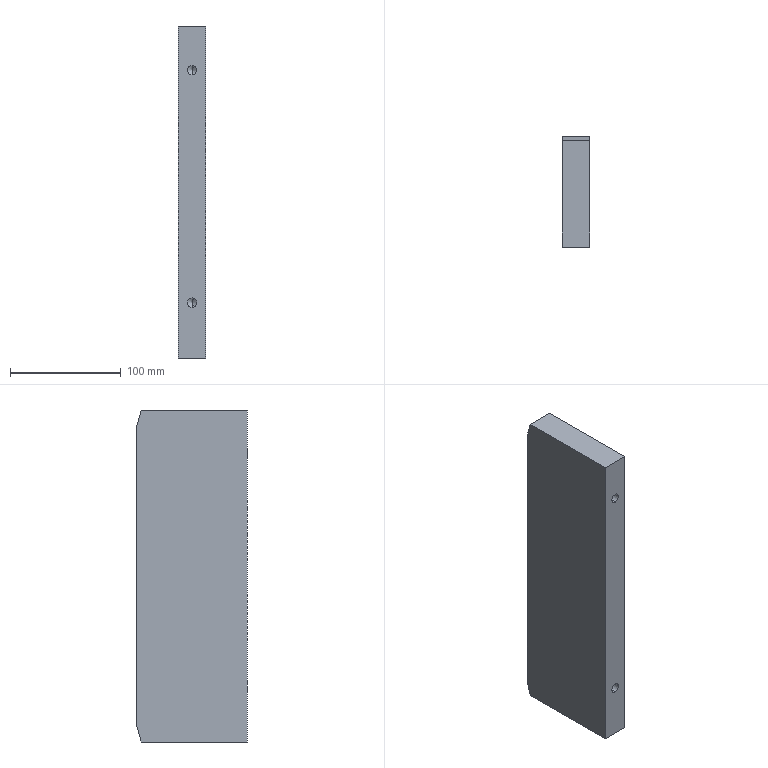Part | STEP file | OP10-033_setup guide  | 1 solid | 16 faces | box 25 x 100 x 300 mm | volume 745616 mm3 | plane 8 | cylinder 4 | cone 4 | commonest cylinder face diameters 8.5 x4
STEP:
#1=CARTESIAN_POINT('',(0.,0.,0.));
#2=DIRECTION('',(0.,0.,1.));
#3=DIRECTION('',(1.,0.,0.));
#4=AXIS2_PLACEMENT_3D('',#1,#2,#3);
#5=CARTESIAN_POINT('',(12.5,24.5,-44.25));
#6=VERTEX_POINT('',#5);
#7=CARTESIAN_POINT('',(12.5,0.,-44.25));
#8=VERTEX_POINT('',#7);
#9=CARTESIAN_POINT('',(12.5,0.,-44.25));
#10=DIRECTION('',(0.,-1.,0.));
#11=VECTOR('',#10,1.);
#12=LINE('',#9,#11);
#13=CARTESIAN_POINT('',(12.5,0.,-40.));
#14=DIRECTION('',(0.,-1.,0.));
#15=DIRECTION('',(0.,0.,-1.));
#16=AXIS2_PLACEMENT_3D('',#13,#14,#15);
#17=CYLINDRICAL_SURFACE('',#16,4.25);
#18=CARTESIAN_POINT('',(6.283,0.));
#19=DIRECTION('',(0.,1.));
#20=VECTOR('',#19,1.);
#21=LINE('',#18,#20);
#22=(GEOMETRIC_REPRESENTATION_CONTEXT(2)PARAMETRIC_REPRESENTATION_CONTEXT()REPRESENTATION_CONTEXT('',''));
#23=DEFINITIONAL_REPRESENTATION('',(#21),#22);
#24=PCURVE('',#17,#23);
#25=CARTESIAN_POINT('',(12.5,0.,-40.));
#26=DIRECTION('',(0.,-1.,0.));
#27=DIRECTION('',(0.,0.,-1.));
#28=AXIS2_PLACEMENT_3D('',#25,#26,#27);
#29=CYLINDRICAL_SURFACE('',#28,4.25);
#30=CARTESIAN_POINT('',(0.,0.));
#31=DIRECTION('',(0.,1.));
#32=VECTOR('',#31,1.);
#33=LINE('',#30,#32);
#34=(GEOMETRIC_REPRESENTATION_CONTEXT(2)PARAMETRIC_REPRESENTATION_CONTEXT()REPRESENTATION_CONTEXT('',''));
#35=DEFINITIONAL_REPRESENTATION('',(#33),#34);
#36=PCURVE('',#29,#35);
#37=SURFACE_CURVE('',#12,(#24,#36),.PCURVE_S1.);
#38=EDGE_CURVE('',#6,#8,#37,.T.);
#39=ORIENTED_EDGE('',*,*,#38,.T.);
#40=CARTESIAN_POINT('',(12.5,0.,-35.75));
#41=VERTEX_POINT('',#40);
#42=CARTESIAN_POINT('',(12.5,0.,-40.));
#43=DIRECTION('',(0.,-1.,0.));
#44=DIRECTION('',(0.,0.,-1.));
#45=AXIS2_PLACEMENT_3D('',#42,#43,#44);
#46=CIRCLE('',#45,4.25);
#47=CARTESIAN_POINT('',(0.,0.));
#48=DIRECTION('',(1.,0.));
#49=VECTOR('',#48,1.);
#50=LINE('',#47,#49);
#51=(GEOMETRIC_REPRESENTATION_CONTEXT(2)PARAMETRIC_REPRESENTATION_CONTEXT()REPRESENTATION_CONTEXT('',''));
#52=DEFINITIONAL_REPRESENTATION('',(#50),#51);
#53=PCURVE('',#17,#52);
#54=CARTESIAN_POINT('',(25.,0.,0.));
#55=DIRECTION('',(0.,1.,0.));
#56=DIRECTION('',(0.,0.,1.));
#57=AXIS2_PLACEMENT_3D('',#54,#55,#56);
#58=PLANE('',#57);
#59=CARTESIAN_POINT('',(-44.25,-12.5));
#60=CARTESIAN_POINT('',(-44.25,-5.139));
#61=CARTESIAN_POINT('',(-37.875,-8.819));
#62=CARTESIAN_POINT('',(-31.5,-12.5));
#63=CARTESIAN_POINT('',(-37.875,-16.181));
#64=CARTESIAN_POINT('',(-44.25,-19.861));
#65=CARTESIAN_POINT('',(-44.25,-12.5));
#66=(BOUNDED_CURVE()B_SPLINE_CURVE(2,(#59,#60,#61,#62,#63,#64,#65),.UNSPECIFIED.,.T.,.F.)B_SPLINE_CURVE_WITH_KNOTS((1,2,2,2,2,1),(-2.094,0.,2.094,4.189,6.283,8.378),.UNSPECIFIED.)CURVE()GEOMETRIC_REPRESENTATION_ITEM()RATIONAL_B_SPLINE_CURVE((1.,0.5,1.,0.5,1.,0.5,1.))REPRESENTATION_ITEM(''));
#67=(GEOMETRIC_REPRESENTATION_CONTEXT(2)PARAMETRIC_REPRESENTATION_CONTEXT()REPRESENTATION_CONTEXT('',''));
#68=DEFINITIONAL_REPRESENTATION('',(#66),#67);
#69=PCURVE('',#58,#68);
#70=SURFACE_CURVE('',#46,(#53,#69),.PCURVE_S1.);
#71=EDGE_CURVE('',#41,#8,#70,.T.);
#72=ORIENTED_EDGE('',*,*,#71,.F.);
#73=CARTESIAN_POINT('',(12.5,24.5,-35.75));
#74=VERTEX_POINT('',#73);
#75=CARTESIAN_POINT('',(12.5,0.,-35.75));
#76=DIRECTION('',(0.,-1.,0.));
#77=VECTOR('',#76,1.);
#78=LINE('',#75,#77);
#79=CARTESIAN_POINT('',(3.142,0.));
#80=DIRECTION('',(0.,1.));
#81=VECTOR('',#80,1.);
#82=LINE('',#79,#81);
#83=(GEOMETRIC_REPRESENTATION_CONTEXT(2)PARAMETRIC_REPRESENTATION_CONTEXT()REPRESENTATION_CONTEXT('',''));
#84=DEFINITIONAL_REPRESENTATION('',(#82),#83);
#85=PCURVE('',#17,#84);
#86=CARTESIAN_POINT('',(3.142,0.));
#87=DIRECTION('',(0.,1.));
#88=VECTOR('',#87,1.);
#89=LINE('',#86,#88);
#90=(GEOMETRIC_REPRESENTATION_CONTEXT(2)PARAMETRIC_REPRESENTATION_CONTEXT()REPRESENTATION_CONTEXT('',''));
#91=DEFINITIONAL_REPRESENTATION('',(#89),#90);
#92=PCURVE('',#29,#91);
#93=SURFACE_CURVE('',#78,(#85,#92),.PCURVE_S1.);
#94=EDGE_CURVE('',#74,#41,#93,.T.);
#95=ORIENTED_EDGE('',*,*,#94,.F.);
#96=CARTESIAN_POINT('',(12.5,24.5,-40.));
#97=DIRECTION('',(0.,-1.,0.));
#98=DIRECTION('',(0.,0.,-1.));
#99=AXIS2_PLACEMENT_3D('',#96,#97,#98);
#100=CIRCLE('',#99,4.25);
#101=CARTESIAN_POINT('',(0.,-24.5));
#102=DIRECTION('',(1.,0.));
#103=VECTOR('',#102,1.);
#104=LINE('',#101,#103);
#105=(GEOMETRIC_REPRESENTATION_CONTEXT(2)PARAMETRIC_REPRESENTATION_CONTEXT()REPRESENTATION_CONTEXT('',''));
#106=DEFINITIONAL_REPRESENTATION('',(#104),#105);
#107=PCURVE('',#17,#106);
#108=CARTESIAN_POINT('',(12.5,24.5,-40.));
#109=DIRECTION('',(0.,-1.,0.));
#110=DIRECTION('',(0.,0.,-1.));
#111=AXIS2_PLACEMENT_3D('',#108,#109,#110);
#112=CONICAL_SURFACE('',#111,4.25,1.03);
#113=CARTESIAN_POINT('',(0.,0.));
#114=DIRECTION('',(1.,0.));
#115=VECTOR('',#114,1.);
#116=LINE('',#113,#115);
#117=(GEOMETRIC_REPRESENTATION_CONTEXT(2)PARAMETRIC_REPRESENTATION_CONTEXT()REPRESENTATION_CONTEXT('',''));
#118=DEFINITIONAL_REPRESENTATION('',(#116),#117);
#119=PCURVE('',#112,#118);
#120=SURFACE_CURVE('',#100,(#107,#119),.PCURVE_S1.);
#121=EDGE_CURVE('',#74,#6,#120,.T.);
#122=ORIENTED_EDGE('',*,*,#121,.T.);
#123=EDGE_LOOP('',(#39,#72,#95,#122));
#124=FACE_BOUND('',#123,.F.);
#125=ADVANCED_FACE('',(#124),#17,.F.);
#126=ORIENTED_EDGE('',*,*,#121,.F.);
#127=CARTESIAN_POINT('',(12.5,27.054,-40.));
#128=VERTEX_POINT('',#127);
#129=CARTESIAN_POINT('',(12.5,24.5,-35.75));
#130=DIRECTION('',(0.,-0.515,0.8572));
#131=VECTOR('',#130,1.);
#132=LINE('',#129,#131);
#133=CARTESIAN_POINT('',(3.142,0.));
#134=DIRECTION('',(0.,1.));
#135=VECTOR('',#134,1.);
#136=LINE('',#133,#135);
#137=(GEOMETRIC_REPRESENTATION_CONTEXT(2)PARAMETRIC_REPRESENTATION_CONTEXT()REPRESENTATION_CONTEXT('',''));
#138=DEFINITIONAL_REPRESENTATION('',(#136),#137);
#139=PCURVE('',#112,#138);
#140=CARTESIAN_POINT('',(12.5,24.5,-40.));
#141=DIRECTION('',(0.,-1.,0.));
#142=DIRECTION('',(0.,0.,-1.));
#143=AXIS2_PLACEMENT_3D('',#140,#141,#142);
#144=CONICAL_SURFACE('',#143,4.25,1.03);
#145=CARTESIAN_POINT('',(3.142,0.));
#146=DIRECTION('',(0.,1.));
#147=VECTOR('',#146,1.);
#148=LINE('',#145,#147);
#149=(GEOMETRIC_REPRESENTATION_CONTEXT(2)PARAMETRIC_REPRESENTATION_CONTEXT()REPRESENTATION_CONTEXT('',''));
#150=DEFINITIONAL_REPRESENTATION('',(#148),#149);
#151=PCURVE('',#144,#150);
#152=SURFACE_CURVE('',#132,(#139,#151),.PCURVE_S1.);
#153=EDGE_CURVE('',#128,#74,#152,.T.);
#154=ORIENTED_EDGE('',*,*,#153,.F.);
#155=CARTESIAN_POINT('',(12.5,24.5,-44.25));
#156=DIRECTION('',(0.,-0.515,-0.8572));
#157=VECTOR('',#156,1.);
#158=LINE('',#155,#157);
#159=CARTESIAN_POINT('',(6.283,0.));
#160=DIRECTION('',(0.,1.));
#161=VECTOR('',#160,1.);
#162=LINE('',#159,#161);
#163=(GEOMETRIC_REPRESENTATION_CONTEXT(2)PARAMETRIC_REPRESENTATION_CONTEXT()REPRESENTATION_CONTEXT('',''));
#164=DEFINITIONAL_REPRESENTATION('',(#162),#163);
#165=PCURVE('',#112,#164);
#166=CARTESIAN_POINT('',(0.,0.));
#167=DIRECTION('',(0.,1.));
#168=VECTOR('',#167,1.);
#169=LINE('',#166,#168);
#170=(GEOMETRIC_REPRESENTATION_CONTEXT(2)PARAMETRIC_REPRESENTATION_CONTEXT()REPRESENTATION_CONTEXT('',''));
#171=DEFINITIONAL_REPRESENTATION('',(#169),#170);
#172=PCURVE('',#144,#171);
#173=SURFACE_CURVE('',#158,(#165,#172),.PCURVE_S1.);
#174=EDGE_CURVE('',#128,#6,#173,.T.);
#175=ORIENTED_EDGE('',*,*,#174,.T.);
#176=EDGE_LOOP('',(#126,#154,#175));
#177=FACE_BOUND('',#176,.F.);
#178=ADVANCED_FACE('',(#177),#112,.F.);
#179=CARTESIAN_POINT('',(12.5,24.5,-254.25));
#180=VERTEX_POINT('',#179);
#181=CARTESIAN_POINT('',(12.5,0.,-254.25));
#182=VERTEX_POINT('',#181);
#183=CARTESIAN_POINT('',(12.5,0.,-254.25));
#184=DIRECTION('',(0.,-1.,0.));
#185=VECTOR('',#184,1.);
#186=LINE('',#183,#185);
#187=CARTESIAN_POINT('',(12.5,0.,-250.));
#188=DIRECTION('',(0.,-1.,0.));
#189=DIRECTION('',(0.,0.,-1.));
#190=AXIS2_PLACEMENT_3D('',#187,#188,#189);
#191=CYLINDRICAL_SURFACE('',#190,4.25);
#192=CARTESIAN_POINT('',(6.283,0.));
#193=DIRECTION('',(0.,1.));
#194=VECTOR('',#193,1.);
#195=LINE('',#192,#194);
#196=(GEOMETRIC_REPRESENTATION_CONTEXT(2)PARAMETRIC_REPRESENTATION_CONTEXT()REPRESENTATION_CONTEXT('',''));
#197=DEFINITIONAL_REPRESENTATION('',(#195),#196);
#198=PCURVE('',#191,#197);
#199=CARTESIAN_POINT('',(12.5,0.,-250.));
#200=DIRECTION('',(0.,-1.,0.));
#201=DIRECTION('',(0.,0.,-1.));
#202=AXIS2_PLACEMENT_3D('',#199,#200,#201);
#203=CYLINDRICAL_SURFACE('',#202,4.25);
#204=CARTESIAN_POINT('',(0.,0.));
#205=DIRECTION('',(0.,1.));
#206=VECTOR('',#205,1.);
#207=LINE('',#204,#206);
#208=(GEOMETRIC_REPRESENTATION_CONTEXT(2)PARAMETRIC_REPRESENTATION_CONTEXT()REPRESENTATION_CONTEXT('',''));
#209=DEFINITIONAL_REPRESENTATION('',(#207),#208);
#210=PCURVE('',#203,#209);
#211=SURFACE_CURVE('',#186,(#198,#210),.PCURVE_S1.);
#212=EDGE_CURVE('',#180,#182,#211,.T.);
#213=ORIENTED_EDGE('',*,*,#212,.T.);
#214=CARTESIAN_POINT('',(12.5,0.,-245.75));
#215=VERTEX_POINT('',#214);
#216=CARTESIAN_POINT('',(12.5,0.,-250.));
#217=DIRECTION('',(0.,-1.,0.));
#218=DIRECTION('',(0.,0.,-1.));
#219=AXIS2_PLACEMENT_3D('',#216,#217,#218);
#220=CIRCLE('',#219,4.25);
#221=CARTESIAN_POINT('',(0.,0.));
#222=DIRECTION('',(1.,0.));
#223=VECTOR('',#222,1.);
#224=LINE('',#221,#223);
#225=(GEOMETRIC_REPRESENTATION_CONTEXT(2)PARAMETRIC_REPRESENTATION_CONTEXT()REPRESENTATION_CONTEXT('',''));
#226=DEFINITIONAL_REPRESENTATION('',(#224),#225);
#227=PCURVE('',#191,#226);
#228=CARTESIAN_POINT('',(-254.25,-12.5));
#229=CARTESIAN_POINT('',(-254.25,-5.139));
#230=CARTESIAN_POINT('',(-247.875,-8.819));
#231=CARTESIAN_POINT('',(-241.5,-12.5));
#232=CARTESIAN_POINT('',(-247.875,-16.181));
#233=CARTESIAN_POINT('',(-254.25,-19.861));
#234=CARTESIAN_POINT('',(-254.25,-12.5));
#235=(BOUNDED_CURVE()B_SPLINE_CURVE(2,(#228,#229,#230,#231,#232,#233,#234),.UNSPECIFIED.,.T.,.F.)B_SPLINE_CURVE_WITH_KNOTS((1,2,2,2,2,1),(-2.094,0.,2.094,4.189,6.283,8.378),.UNSPECIFIED.)CURVE()GEOMETRIC_REPRESENTATION_ITEM()RATIONAL_B_SPLINE_CURVE((1.,0.5,1.,0.5,1.,0.5,1.))REPRESENTATION_ITEM(''));
#236=(GEOMETRIC_REPRESENTATION_CONTEXT(2)PARAMETRIC_REPRESENTATION_CONTEXT()REPRESENTATION_CONTEXT('',''));
#237=DEFINITIONAL_REPRESENTATION('',(#235),#236);
#238=PCURVE('',#58,#237);
#239=SURFACE_CURVE('',#220,(#227,#238),.PCURVE_S1.);
#240=EDGE_CURVE('',#215,#182,#239,.T.);
#241=ORIENTED_EDGE('',*,*,#240,.F.);
#242=CARTESIAN_POINT('',(12.5,24.5,-245.75));
#243=VERTEX_POINT('',#242);
#244=CARTESIAN_POINT('',(12.5,0.,-245.75));
#245=DIRECTION('',(0.,-1.,0.));
#246=VECTOR('',#245,1.);
#247=LINE('',#244,#246);
#248=CARTESIAN_POINT('',(3.142,0.));
#249=DIRECTION('',(0.,1.));
#250=VECTOR('',#249,1.);
#251=LINE('',#248,#250);
#252=(GEOMETRIC_REPRESENTATION_CONTEXT(2)PARAMETRIC_REPRESENTATION_CONTEXT()REPRESENTATION_CONTEXT('',''));
#253=DEFINITIONAL_REPRESENTATION('',(#251),#252);
#254=PCURVE('',#191,#253);
#255=CARTESIAN_POINT('',(3.142,0.));
#256=DIRECTION('',(0.,1.));
#257=VECTOR('',#256,1.);
#258=LINE('',#255,#257);
#259=(GEOMETRIC_REPRESENTATION_CONTEXT(2)PARAMETRIC_REPRESENTATION_CONTEXT()REPRESENTATION_CONTEXT('',''));
#260=DEFINITIONAL_REPRESENTATION('',(#258),#259);
#261=PCURVE('',#203,#260);
#262=SURFACE_CURVE('',#247,(#254,#261),.PCURVE_S1.);
#263=EDGE_CURVE('',#243,#215,#262,.T.);
#264=ORIENTED_EDGE('',*,*,#263,.F.);
#265=CARTESIAN_POINT('',(12.5,24.5,-250.));
#266=DIRECTION('',(0.,-1.,0.));
#267=DIRECTION('',(0.,0.,-1.));
#268=AXIS2_PLACEMENT_3D('',#265,#266,#267);
#269=CIRCLE('',#268,4.25);
#270=CARTESIAN_POINT('',(0.,-24.5));
#271=DIRECTION('',(1.,0.));
#272=VECTOR('',#271,1.);
#273=LINE('',#270,#272);
#274=(GEOMETRIC_REPRESENTATION_CONTEXT(2)PARAMETRIC_REPRESENTATION_CONTEXT()REPRESENTATION_CONTEXT('',''));
#275=DEFINITIONAL_REPRESENTATION('',(#273),#274);
#276=PCURVE('',#191,#275);
#277=CARTESIAN_POINT('',(12.5,24.5,-250.));
#278=DIRECTION('',(0.,-1.,0.));
#279=DIRECTION('',(0.,0.,-1.));
#280=AXIS2_PLACEMENT_3D('',#277,#278,#279);
#281=CONICAL_SURFACE('',#280,4.25,1.03);
#282=CARTESIAN_POINT('',(0.,0.));
#283=DIRECTION('',(1.,0.));
#284=VECTOR('',#283,1.);
#285=LINE('',#282,#284);
#286=(GEOMETRIC_REPRESENTATION_CONTEXT(2)PARAMETRIC_REPRESENTATION_CONTEXT()REPRESENTATION_CONTEXT('',''));
#287=DEFINITIONAL_REPRESENTATION('',(#285),#286);
#288=PCURVE('',#281,#287);
#289=SURFACE_CURVE('',#269,(#276,#288),.PCURVE_S1.);
#290=EDGE_CURVE('',#243,#180,#289,.T.);
#291=ORIENTED_EDGE('',*,*,#290,.T.);
#292=EDGE_LOOP('',(#213,#241,#264,#291));
#293=FACE_BOUND('',#292,.F.);
#294=ADVANCED_FACE('',(#293),#191,.F.);
#295=ORIENTED_EDGE('',*,*,#290,.F.);
#296=CARTESIAN_POINT('',(12.5,27.054,-250.));
#297=VERTEX_POINT('',#296);
#298=CARTESIAN_POINT('',(12.5,24.5,-245.75));
#299=DIRECTION('',(0.,-0.515,0.8572));
#300=VECTOR('',#299,1.);
#301=LINE('',#298,#300);
#302=CARTESIAN_POINT('',(3.142,-2.554));
#303=CARTESIAN_POINT('',(3.142,-2.515));
#304=CARTESIAN_POINT('',(3.142,-2.438));
#305=CARTESIAN_POINT('',(3.142,-2.322));
#306=CARTESIAN_POINT('',(3.142,-2.205));
#307=CARTESIAN_POINT('',(3.142,-2.089));
#308=CARTESIAN_POINT('',(3.142,-1.973));
#309=CARTESIAN_POINT('',(3.142,-1.857));
#310=CARTESIAN_POINT('',(3.142,-1.741));
#311=CARTESIAN_POINT('',(3.142,-1.625));
#312=CARTESIAN_POINT('',(3.142,-1.509));
#313=CARTESIAN_POINT('',(3.142,-1.393));
#314=CARTESIAN_POINT('',(3.142,-1.277));
#315=CARTESIAN_POINT('',(3.142,-1.161));
#316=CARTESIAN_POINT('',(3.142,-1.045));
#317=CARTESIAN_POINT('',(3.142,-0.9286));
#318=CARTESIAN_POINT('',(3.142,-0.8125));
#319=CARTESIAN_POINT('',(3.142,-0.6965));
#320=CARTESIAN_POINT('',(3.142,-0.5804));
#321=CARTESIAN_POINT('',(3.142,-0.4643));
#322=CARTESIAN_POINT('',(3.142,-0.3482));
#323=CARTESIAN_POINT('',(3.142,-0.2322));
#324=CARTESIAN_POINT('',(3.142,-0.1161));
#325=CARTESIAN_POINT('',(3.142,-0.03869));
#326=CARTESIAN_POINT('',(3.142,0.));
#327=B_SPLINE_CURVE_WITH_KNOTS('',3,(#302,#303,#304,#305,#306,#307,#308,#309,#310,#311,#312,#313,#314,#315,#316,#317,#318,#319,#320,#321,#322,#323,#324,#325,#326),.UNSPECIFIED.,.F.,.F.,(4,1,1,1,1,1,1,1,1,1,1,1,1,1,1,1,1,1,1,1,1,1,4),(-4.958,-4.733,-4.507,-4.282,-4.057,-3.831,-3.606,-3.381,-3.155,-2.93,-2.704,-2.479,-2.254,-2.028,-1.803,-1.578,-1.352,-1.127,-0.9015,-0.6761,-0.4507,-0.2254,0.),.QUASI_UNIFORM_KNOTS.);
#328=(GEOMETRIC_REPRESENTATION_CONTEXT(2)PARAMETRIC_REPRESENTATION_CONTEXT()REPRESENTATION_CONTEXT('',''));
#329=DEFINITIONAL_REPRESENTATION('',(#327),#328);
#330=PCURVE('',#281,#329);
#331=CARTESIAN_POINT('',(12.5,24.5,-250.));
#332=DIRECTION('',(0.,-1.,0.));
#333=DIRECTION('',(0.,0.,-1.));
#334=AXIS2_PLACEMENT_3D('',#331,#332,#333);
#335=CONICAL_SURFACE('',#334,4.25,1.03);
#336=CARTESIAN_POINT('',(3.142,-2.554));
#337=CARTESIAN_POINT('',(3.142,-2.515));
#338=CARTESIAN_POINT('',(3.142,-2.438));
#339=CARTESIAN_POINT('',(3.142,-2.322));
#340=CARTESIAN_POINT('',(3.142,-2.205));
#341=CARTESIAN_POINT('',(3.142,-2.089));
#342=CARTESIAN_POINT('',(3.142,-1.973));
#343=CARTESIAN_POINT('',(3.142,-1.857));
#344=CARTESIAN_POINT('',(3.142,-1.741));
#345=CARTESIAN_POINT('',(3.142,-1.625));
#346=CARTESIAN_POINT('',(3.142,-1.509));
#347=CARTESIAN_POINT('',(3.142,-1.393));
#348=CARTESIAN_POINT('',(3.142,-1.277));
#349=CARTESIAN_POINT('',(3.142,-1.161));
#350=CARTESIAN_POINT('',(3.142,-1.045));
#351=CARTESIAN_POINT('',(3.142,-0.9286));
#352=CARTESIAN_POINT('',(3.142,-0.8125));
#353=CARTESIAN_POINT('',(3.142,-0.6965));
#354=CARTESIAN_POINT('',(3.142,-0.5804));
#355=CARTESIAN_POINT('',(3.142,-0.4643));
#356=CARTESIAN_POINT('',(3.142,-0.3482));
#357=CARTESIAN_POINT('',(3.142,-0.2322));
#358=CARTESIAN_POINT('',(3.142,-0.1161));
#359=CARTESIAN_POINT('',(3.142,-0.03869));
#360=CARTESIAN_POINT('',(3.142,0.));
#361=B_SPLINE_CURVE_WITH_KNOTS('',3,(#336,#337,#338,#339,#340,#341,#342,#343,#344,#345,#346,#347,#348,#349,#350,#351,#352,#353,#354,#355,#356,#357,#358,#359,#360),.UNSPECIFIED.,.F.,.F.,(4,1,1,1,1,1,1,1,1,1,1,1,1,1,1,1,1,1,1,1,1,1,4),(-4.958,-4.733,-4.507,-4.282,-4.057,-3.831,-3.606,-3.381,-3.155,-2.93,-2.704,-2.479,-2.254,-2.028,-1.803,-1.578,-1.352,-1.127,-0.9015,-0.6761,-0.4507,-0.2254,0.),.QUASI_UNIFORM_KNOTS.);
#362=(GEOMETRIC_REPRESENTATION_CONTEXT(2)PARAMETRIC_REPRESENTATION_CONTEXT()REPRESENTATION_CONTEXT('',''));
#363=DEFINITIONAL_REPRESENTATION('',(#361),#362);
#364=PCURVE('',#335,#363);
#365=SURFACE_CURVE('',#301,(#330,#364),.PCURVE_S1.);
#366=EDGE_CURVE('',#297,#243,#365,.T.);
#367=ORIENTED_EDGE('',*,*,#366,.F.);
#368=CARTESIAN_POINT('',(12.5,24.5,-254.25));
#369=DIRECTION('',(0.,-0.515,-0.8572));
#370=VECTOR('',#369,1.);
#371=LINE('',#368,#370);
#372=CARTESIAN_POINT('',(6.283,0.));
#373=DIRECTION('',(0.,1.));
#374=VECTOR('',#373,1.);
#375=LINE('',#372,#374);
#376=(GEOMETRIC_REPRESENTATION_CONTEXT(2)PARAMETRIC_REPRESENTATION_CONTEXT()REPRESENTATION_CONTEXT('',''));
#377=DEFINITIONAL_REPRESENTATION('',(#375),#376);
#378=PCURVE('',#281,#377);
#379=CARTESIAN_POINT('',(0.,0.));
#380=DIRECTION('',(0.,1.));
#381=VECTOR('',#380,1.);
#382=LINE('',#379,#381);
#383=(GEOMETRIC_REPRESENTATION_CONTEXT(2)PARAMETRIC_REPRESENTATION_CONTEXT()REPRESENTATION_CONTEXT('',''));
#384=DEFINITIONAL_REPRESENTATION('',(#382),#383);
#385=PCURVE('',#335,#384);
#386=SURFACE_CURVE('',#371,(#378,#385),.PCURVE_S1.);
#387=EDGE_CURVE('',#297,#180,#386,.T.);
#388=ORIENTED_EDGE('',*,*,#387,.T.);
#389=EDGE_LOOP('',(#295,#367,#388));
#390=FACE_BOUND('',#389,.F.);
#391=ADVANCED_FACE('',(#390),#281,.F.);
#392=CARTESIAN_POINT('',(0.,95.981,0.));
#393=VERTEX_POINT('',#392);
#394=CARTESIAN_POINT('',(0.,0.,0.));
#395=VERTEX_POINT('',#394);
#396=CARTESIAN_POINT('',(0.,0.,0.));
#397=DIRECTION('',(0.,-1.,0.));
#398=VECTOR('',#397,1.);
#399=LINE('',#396,#398);
#400=CARTESIAN_POINT('',(25.,0.,0.));
#401=DIRECTION('',(0.,0.,-1.));
#402=DIRECTION('',(-1.,0.,0.));
#403=AXIS2_PLACEMENT_3D('',#400,#401,#402);
#404=PLANE('',#403);
#405=CARTESIAN_POINT('',(25.,0.));
#406=DIRECTION('',(0.,-1.));
#407=VECTOR('',#406,1.);
#408=LINE('',#405,#407);
#409=(GEOMETRIC_REPRESENTATION_CONTEXT(2)PARAMETRIC_REPRESENTATION_CONTEXT()REPRESENTATION_CONTEXT('',''));
#410=DEFINITIONAL_REPRESENTATION('',(#408),#409);
#411=PCURVE('',#404,#410);
#412=CARTESIAN_POINT('',(0.,100.,0.));
#413=DIRECTION('',(-1.,0.,0.));
#414=DIRECTION('',(0.,0.,1.));
#415=AXIS2_PLACEMENT_3D('',#412,#413,#414);
#416=PLANE('',#415);
#417=CARTESIAN_POINT('',(0.,-100.));
#418=DIRECTION('',(0.,-1.));
#419=VECTOR('',#418,1.);
#420=LINE('',#417,#419);
#421=(GEOMETRIC_REPRESENTATION_CONTEXT(2)PARAMETRIC_REPRESENTATION_CONTEXT()REPRESENTATION_CONTEXT('',''));
#422=DEFINITIONAL_REPRESENTATION('',(#420),#421);
#423=PCURVE('',#416,#422);
#424=SURFACE_CURVE('',#399,(#411,#423),.PCURVE_S1.);
#425=EDGE_CURVE('',#393,#395,#424,.T.);
#426=ORIENTED_EDGE('',*,*,#425,.T.);
#427=CARTESIAN_POINT('',(25.,0.,0.));
#428=VERTEX_POINT('',#427);
#429=CARTESIAN_POINT('',(25.,0.,0.));
#430=DIRECTION('',(-1.,0.,0.));
#431=VECTOR('',#430,1.);
#432=LINE('',#429,#431);
#433=CARTESIAN_POINT('',(0.,0.));
#434=DIRECTION('',(1.,0.));
#435=VECTOR('',#434,1.);
#436=LINE('',#433,#435);
#437=(GEOMETRIC_REPRESENTATION_CONTEXT(2)PARAMETRIC_REPRESENTATION_CONTEXT()REPRESENTATION_CONTEXT('',''));
#438=DEFINITIONAL_REPRESENTATION('',(#436),#437);
#439=PCURVE('',#404,#438);
#440=CARTESIAN_POINT('',(0.,0.));
#441=DIRECTION('',(0.,-1.));
#442=VECTOR('',#441,1.);
#443=LINE('',#440,#442);
#444=(GEOMETRIC_REPRESENTATION_CONTEXT(2)PARAMETRIC_REPRESENTATION_CONTEXT()REPRESENTATION_CONTEXT('',''));
#445=DEFINITIONAL_REPRESENTATION('',(#443),#444);
#446=PCURVE('',#58,#445);
#447=SURFACE_CURVE('',#432,(#439,#446),.PCURVE_S1.);
#448=EDGE_CURVE('',#428,#395,#447,.T.);
#449=ORIENTED_EDGE('',*,*,#448,.F.);
#450=CARTESIAN_POINT('',(25.,95.981,0.));
#451=VERTEX_POINT('',#450);
#452=CARTESIAN_POINT('',(25.,0.,0.));
#453=DIRECTION('',(0.,-1.,0.));
#454=VECTOR('',#453,1.);
#455=LINE('',#452,#454);
#456=CARTESIAN_POINT('',(0.,0.));
#457=DIRECTION('',(0.,-1.));
#458=VECTOR('',#457,1.);
#459=LINE('',#456,#458);
#460=(GEOMETRIC_REPRESENTATION_CONTEXT(2)PARAMETRIC_REPRESENTATION_CONTEXT()REPRESENTATION_CONTEXT('',''));
#461=DEFINITIONAL_REPRESENTATION('',(#459),#460);
#462=PCURVE('',#404,#461);
#463=CARTESIAN_POINT('',(25.,100.,0.));
#464=DIRECTION('',(-1.,0.,0.));
#465=DIRECTION('',(0.,0.,1.));
#466=AXIS2_PLACEMENT_3D('',#463,#464,#465);
#467=PLANE('',#466);
#468=CARTESIAN_POINT('',(0.,-100.));
#469=DIRECTION('',(0.,-1.));
#470=VECTOR('',#469,1.);
#471=LINE('',#468,#470);
#472=(GEOMETRIC_REPRESENTATION_CONTEXT(2)PARAMETRIC_REPRESENTATION_CONTEXT()REPRESENTATION_CONTEXT('',''));
#473=DEFINITIONAL_REPRESENTATION('',(#471),#472);
#474=PCURVE('',#467,#473);
#475=SURFACE_CURVE('',#455,(#462,#474),.PCURVE_S1.);
#476=EDGE_CURVE('',#451,#428,#475,.T.);
#477=ORIENTED_EDGE('',*,*,#476,.F.);
#478=CARTESIAN_POINT('',(25.,95.981,0.));
#479=DIRECTION('',(-1.,0.,0.));
#480=VECTOR('',#479,1.);
#481=LINE('',#478,#480);
#482=CARTESIAN_POINT('',(0.,95.981));
#483=DIRECTION('',(1.,0.));
#484=VECTOR('',#483,1.);
#485=LINE('',#482,#484);
#486=(GEOMETRIC_REPRESENTATION_CONTEXT(2)PARAMETRIC_REPRESENTATION_CONTEXT()REPRESENTATION_CONTEXT('',''));
#487=DEFINITIONAL_REPRESENTATION('',(#485),#486);
#488=PCURVE('',#404,#487);
#489=CARTESIAN_POINT('',(25.,95.981,0.));
#490=DIRECTION('',(0.,-0.9659,-0.2588));
#491=DIRECTION('',(0.,0.2588,-0.9659));
#492=AXIS2_PLACEMENT_3D('',#489,#490,#491);
#493=PLANE('',#492);
#494=CARTESIAN_POINT('',(0.,0.));
#495=DIRECTION('',(0.,-1.));
#496=VECTOR('',#495,1.);
#497=LINE('',#494,#496);
#498=(GEOMETRIC_REPRESENTATION_CONTEXT(2)PARAMETRIC_REPRESENTATION_CONTEXT()REPRESENTATION_CONTEXT('',''));
#499=DEFINITIONAL_REPRESENTATION('',(#497),#498);
#500=PCURVE('',#493,#499);
#501=SURFACE_CURVE('',#481,(#488,#500),.PCURVE_S1.);
#502=EDGE_CURVE('',#451,#393,#501,.T.);
#503=ORIENTED_EDGE('',*,*,#502,.T.);
#504=EDGE_LOOP('',(#426,#449,#477,#503));
#505=FACE_BOUND('',#504,.T.);
#506=ADVANCED_FACE('',(#505),#404,.F.);
#507=CARTESIAN_POINT('',(12.5,0.,-40.));
#508=DIRECTION('',(0.,-1.,0.));
#509=DIRECTION('',(0.,0.,-1.));
#510=AXIS2_PLACEMENT_3D('',#507,#508,#509);
#511=CIRCLE('',#510,4.25);
#512=CARTESIAN_POINT('',(-44.25,-12.5));
#513=CARTESIAN_POINT('',(-44.25,-5.139));
#514=CARTESIAN_POINT('',(-37.875,-8.819));
#515=CARTESIAN_POINT('',(-31.5,-12.5));
#516=CARTESIAN_POINT('',(-37.875,-16.181));
#517=CARTESIAN_POINT('',(-44.25,-19.861));
#518=CARTESIAN_POINT('',(-44.25,-12.5));
#519=(BOUNDED_CURVE()B_SPLINE_CURVE(2,(#512,#513,#514,#515,#516,#517,#518),.UNSPECIFIED.,.T.,.F.)B_SPLINE_CURVE_WITH_KNOTS((1,2,2,2,2,1),(-2.094,0.,2.094,4.189,6.283,8.378),.UNSPECIFIED.)CURVE()GEOMETRIC_REPRESENTATION_ITEM()RATIONAL_B_SPLINE_CURVE((1.,0.5,1.,0.5,1.,0.5,1.))REPRESENTATION_ITEM(''));
#520=(GEOMETRIC_REPRESENTATION_CONTEXT(2)PARAMETRIC_REPRESENTATION_CONTEXT()REPRESENTATION_CONTEXT('',''));
#521=DEFINITIONAL_REPRESENTATION('',(#519),#520);
#522=PCURVE('',#58,#521);
#523=CARTESIAN_POINT('',(0.,0.));
#524=DIRECTION('',(1.,0.));
#525=VECTOR('',#524,1.);
#526=LINE('',#523,#525);
#527=(GEOMETRIC_REPRESENTATION_CONTEXT(2)PARAMETRIC_REPRESENTATION_CONTEXT()REPRESENTATION_CONTEXT('',''));
#528=DEFINITIONAL_REPRESENTATION('',(#526),#527);
#529=PCURVE('',#29,#528);
#530=SURFACE_CURVE('',#511,(#522,#529),.PCURVE_S1.);
#531=EDGE_CURVE('',#8,#41,#530,.T.);
#532=ORIENTED_EDGE('',*,*,#531,.F.);
#533=ORIENTED_EDGE('',*,*,#71,.F.);
#534=EDGE_LOOP('',(#532,#533));
#535=FACE_BOUND('',#534,.T.);
#536=CARTESIAN_POINT('',(12.5,0.,-250.));
#537=DIRECTION('',(0.,-1.,0.));
#538=DIRECTION('',(0.,0.,-1.));
#539=AXIS2_PLACEMENT_3D('',#536,#537,#538);
#540=CIRCLE('',#539,4.25);
#541=CARTESIAN_POINT('',(-254.25,-12.5));
#542=CARTESIAN_POINT('',(-254.25,-5.139));
#543=CARTESIAN_POINT('',(-247.875,-8.819));
#544=CARTESIAN_POINT('',(-241.5,-12.5));
#545=CARTESIAN_POINT('',(-247.875,-16.181));
#546=CARTESIAN_POINT('',(-254.25,-19.861));
#547=CARTESIAN_POINT('',(-254.25,-12.5));
#548=(BOUNDED_CURVE()B_SPLINE_CURVE(2,(#541,#542,#543,#544,#545,#546,#547),.UNSPECIFIED.,.T.,.F.)B_SPLINE_CURVE_WITH_KNOTS((1,2,2,2,2,1),(-2.094,0.,2.094,4.189,6.283,8.378),.UNSPECIFIED.)CURVE()GEOMETRIC_REPRESENTATION_ITEM()RATIONAL_B_SPLINE_CURVE((1.,0.5,1.,0.5,1.,0.5,1.))REPRESENTATION_ITEM(''));
#549=(GEOMETRIC_REPRESENTATION_CONTEXT(2)PARAMETRIC_REPRESENTATION_CONTEXT()REPRESENTATION_CONTEXT('',''));
#550=DEFINITIONAL_REPRESENTATION('',(#548),#549);
#551=PCURVE('',#58,#550);
#552=CARTESIAN_POINT('',(0.,0.));
#553=DIRECTION('',(1.,0.));
#554=VECTOR('',#553,1.);
#555=LINE('',#552,#554);
#556=(GEOMETRIC_REPRESENTATION_CONTEXT(2)PARAMETRIC_REPRESENTATION_CONTEXT()REPRESENTATION_CONTEXT('',''));
#557=DEFINITIONAL_REPRESENTATION('',(#555),#556);
#558=PCURVE('',#203,#557);
#559=SURFACE_CURVE('',#540,(#551,#558),.PCURVE_S1.);
#560=EDGE_CURVE('',#182,#215,#559,.T.);
#561=ORIENTED_EDGE('',*,*,#560,.F.);
#562=ORIENTED_EDGE('',*,*,#240,.F.);
#563=EDGE_LOOP('',(#561,#562));
#564=FACE_BOUND('',#563,.T.);
#565=CARTESIAN_POINT('',(0.,0.,-300.));
#566=VERTEX_POINT('',#565);
#567=CARTESIAN_POINT('',(0.,0.,0.));
#568=DIRECTION('',(0.,0.,-1.));
#569=VECTOR('',#568,1.);
#570=LINE('',#567,#569);
#571=CARTESIAN_POINT('',(0.,-25.));
#572=DIRECTION('',(-1.,0.));
#573=VECTOR('',#572,1.);
#574=LINE('',#571,#573);
#575=(GEOMETRIC_REPRESENTATION_CONTEXT(2)PARAMETRIC_REPRESENTATION_CONTEXT()REPRESENTATION_CONTEXT('',''));
#576=DEFINITIONAL_REPRESENTATION('',(#574),#575);
#577=PCURVE('',#58,#576);
#578=CARTESIAN_POINT('',(0.,-100.));
#579=DIRECTION('',(-1.,0.));
#580=VECTOR('',#579,1.);
#581=LINE('',#578,#580);
#582=(GEOMETRIC_REPRESENTATION_CONTEXT(2)PARAMETRIC_REPRESENTATION_CONTEXT()REPRESENTATION_CONTEXT('',''));
#583=DEFINITIONAL_REPRESENTATION('',(#581),#582);
#584=PCURVE('',#416,#583);
#585=SURFACE_CURVE('',#570,(#577,#584),.PCURVE_S1.);
#586=EDGE_CURVE('',#395,#566,#585,.T.);
#587=ORIENTED_EDGE('',*,*,#586,.T.);
#588=CARTESIAN_POINT('',(25.,0.,-300.));
#589=VERTEX_POINT('',#588);
#590=CARTESIAN_POINT('',(25.,0.,-300.));
#591=DIRECTION('',(-1.,0.,0.));
#592=VECTOR('',#591,1.);
#593=LINE('',#590,#592);
#594=CARTESIAN_POINT('',(-300.,0.));
#595=DIRECTION('',(0.,-1.));
#596=VECTOR('',#595,1.);
#597=LINE('',#594,#596);
#598=(GEOMETRIC_REPRESENTATION_CONTEXT(2)PARAMETRIC_REPRESENTATION_CONTEXT()REPRESENTATION_CONTEXT('',''));
#599=DEFINITIONAL_REPRESENTATION('',(#597),#598);
#600=PCURVE('',#58,#599);
#601=CARTESIAN_POINT('',(25.,0.,-300.));
#602=DIRECTION('',(0.,0.,1.));
#603=DIRECTION('',(0.,-1.,0.));
#604=AXIS2_PLACEMENT_3D('',#601,#602,#603);
#605=PLANE('',#604);
#606=CARTESIAN_POINT('',(0.,0.));
#607=DIRECTION('',(0.,-1.));
#608=VECTOR('',#607,1.);
#609=LINE('',#606,#608);
#610=(GEOMETRIC_REPRESENTATION_CONTEXT(2)PARAMETRIC_REPRESENTATION_CONTEXT()REPRESENTATION_CONTEXT('',''));
#611=DEFINITIONAL_REPRESENTATION('',(#609),#610);
#612=PCURVE('',#605,#611);
#613=SURFACE_CURVE('',#593,(#600,#612),.PCURVE_S1.);
#614=EDGE_CURVE('',#589,#566,#613,.T.);
#615=ORIENTED_EDGE('',*,*,#614,.F.);
#616=CARTESIAN_POINT('',(25.,0.,0.));
#617=DIRECTION('',(0.,0.,-1.));
#618=VECTOR('',#617,1.);
#619=LINE('',#616,#618);
#620=CARTESIAN_POINT('',(0.,0.));
#621=DIRECTION('',(-1.,0.));
#622=VECTOR('',#621,1.);
#623=LINE('',#620,#622);
#624=(GEOMETRIC_REPRESENTATION_CONTEXT(2)PARAMETRIC_REPRESENTATION_CONTEXT()REPRESENTATION_CONTEXT('',''));
#625=DEFINITIONAL_REPRESENTATION('',(#623),#624);
#626=PCURVE('',#58,#625);
#627=CARTESIAN_POINT('',(0.,-100.));
#628=DIRECTION('',(-1.,0.));
#629=VECTOR('',#628,1.);
#630=LINE('',#627,#629);
#631=(GEOMETRIC_REPRESENTATION_CONTEXT(2)PARAMETRIC_REPRESENTATION_CONTEXT()REPRESENTATION_CONTEXT('',''));
#632=DEFINITIONAL_REPRESENTATION('',(#630),#631);
#633=PCURVE('',#467,#632);
#634=SURFACE_CURVE('',#619,(#626,#633),.PCURVE_S1.);
#635=EDGE_CURVE('',#428,#589,#634,.T.);
#636=ORIENTED_EDGE('',*,*,#635,.F.);
#637=ORIENTED_EDGE('',*,*,#448,.T.);
#638=EDGE_LOOP('',(#587,#615,#636,#637));
#639=FACE_BOUND('',#638,.T.);
#640=ADVANCED_FACE('',(#535,#564,#639),#58,.F.);
#641=CARTESIAN_POINT('',(0.,95.981,-300.));
#642=VERTEX_POINT('',#641);
#643=CARTESIAN_POINT('',(0.,0.,-300.));
#644=DIRECTION('',(0.,1.,0.));
#645=VECTOR('',#644,1.);
#646=LINE('',#643,#645);
#647=CARTESIAN_POINT('',(0.,-25.));
#648=DIRECTION('',(-1.,0.));
#649=VECTOR('',#648,1.);
#650=LINE('',#647,#649);
#651=(GEOMETRIC_REPRESENTATION_CONTEXT(2)PARAMETRIC_REPRESENTATION_CONTEXT()REPRESENTATION_CONTEXT('',''));
#652=DEFINITIONAL_REPRESENTATION('',(#650),#651);
#653=PCURVE('',#605,#652);
#654=CARTESIAN_POINT('',(-300.,-100.));
#655=DIRECTION('',(0.,1.));
#656=VECTOR('',#655,1.);
#657=LINE('',#654,#656);
#658=(GEOMETRIC_REPRESENTATION_CONTEXT(2)PARAMETRIC_REPRESENTATION_CONTEXT()REPRESENTATION_CONTEXT('',''));
#659=DEFINITIONAL_REPRESENTATION('',(#657),#658);
#660=PCURVE('',#416,#659);
#661=SURFACE_CURVE('',#646,(#653,#660),.PCURVE_S1.);
#662=EDGE_CURVE('',#566,#642,#661,.T.);
#663=ORIENTED_EDGE('',*,*,#662,.T.);
#664=CARTESIAN_POINT('',(25.,95.981,-300.));
#665=VERTEX_POINT('',#664);
#666=CARTESIAN_POINT('',(25.,95.981,-300.));
#667=DIRECTION('',(-1.,0.,0.));
#668=VECTOR('',#667,1.);
#669=LINE('',#666,#668);
#670=CARTESIAN_POINT('',(-95.981,0.));
#671=DIRECTION('',(0.,-1.));
#672=VECTOR('',#671,1.);
#673=LINE('',#670,#672);
#674=(GEOMETRIC_REPRESENTATION_CONTEXT(2)PARAMETRIC_REPRESENTATION_CONTEXT()REPRESENTATION_CONTEXT('',''));
#675=DEFINITIONAL_REPRESENTATION('',(#673),#674);
#676=PCURVE('',#605,#675);
#677=CARTESIAN_POINT('',(25.,100.,-285.));
#678=DIRECTION('',(0.,-0.9659,0.2588));
#679=DIRECTION('',(0.,-0.2588,-0.9659));
#680=AXIS2_PLACEMENT_3D('',#677,#678,#679);
#681=PLANE('',#680);
#682=CARTESIAN_POINT('',(15.529,0.));
#683=DIRECTION('',(0.,-1.));
#684=VECTOR('',#683,1.);
#685=LINE('',#682,#684);
#686=(GEOMETRIC_REPRESENTATION_CONTEXT(2)PARAMETRIC_REPRESENTATION_CONTEXT()REPRESENTATION_CONTEXT('',''));
#687=DEFINITIONAL_REPRESENTATION('',(#685),#686);
#688=PCURVE('',#681,#687);
#689=SURFACE_CURVE('',#669,(#676,#688),.PCURVE_S1.);
#690=EDGE_CURVE('',#665,#642,#689,.T.);
#691=ORIENTED_EDGE('',*,*,#690,.F.);
#692=CARTESIAN_POINT('',(25.,0.,-300.));
#693=DIRECTION('',(0.,1.,0.));
#694=VECTOR('',#693,1.);
#695=LINE('',#692,#694);
#696=CARTESIAN_POINT('',(0.,0.));
#697=DIRECTION('',(-1.,0.));
#698=VECTOR('',#697,1.);
#699=LINE('',#696,#698);
#700=(GEOMETRIC_REPRESENTATION_CONTEXT(2)PARAMETRIC_REPRESENTATION_CONTEXT()REPRESENTATION_CONTEXT('',''));
#701=DEFINITIONAL_REPRESENTATION('',(#699),#700);
#702=PCURVE('',#605,#701);
#703=CARTESIAN_POINT('',(-300.,-100.));
#704=DIRECTION('',(0.,1.));
#705=VECTOR('',#704,1.);
#706=LINE('',#703,#705);
#707=(GEOMETRIC_REPRESENTATION_CONTEXT(2)PARAMETRIC_REPRESENTATION_CONTEXT()REPRESENTATION_CONTEXT('',''));
#708=DEFINITIONAL_REPRESENTATION('',(#706),#707);
#709=PCURVE('',#467,#708);
#710=SURFACE_CURVE('',#695,(#702,#709),.PCURVE_S1.);
#711=EDGE_CURVE('',#589,#665,#710,.T.);
#712=ORIENTED_EDGE('',*,*,#711,.F.);
#713=ORIENTED_EDGE('',*,*,#614,.T.);
#714=EDGE_LOOP('',(#663,#691,#712,#713));
#715=FACE_BOUND('',#714,.T.);
#716=ADVANCED_FACE('',(#715),#605,.F.);
#717=CARTESIAN_POINT('',(0.,100.,-285.));
#718=VERTEX_POINT('',#717);
#719=CARTESIAN_POINT('',(0.,100.,-285.));
#720=DIRECTION('',(0.,0.2588,0.9659));
#721=VECTOR('',#720,1.);
#722=LINE('',#719,#721);
#723=CARTESIAN_POINT('',(0.,-25.));
#724=DIRECTION('',(-1.,0.));
#725=VECTOR('',#724,1.);
#726=LINE('',#723,#725);
#727=(GEOMETRIC_REPRESENTATION_CONTEXT(2)PARAMETRIC_REPRESENTATION_CONTEXT()REPRESENTATION_CONTEXT('',''));
#728=DEFINITIONAL_REPRESENTATION('',(#726),#727);
#729=PCURVE('',#681,#728);
#730=CARTESIAN_POINT('',(-285.,0.));
#731=DIRECTION('',(0.9659,0.2588));
#732=VECTOR('',#731,1.);
#733=LINE('',#730,#732);
#734=(GEOMETRIC_REPRESENTATION_CONTEXT(2)PARAMETRIC_REPRESENTATION_CONTEXT()REPRESENTATION_CONTEXT('',''));
#735=DEFINITIONAL_REPRESENTATION('',(#733),#734);
#736=PCURVE('',#416,#735);
#737=SURFACE_CURVE('',#722,(#729,#736),.PCURVE_S1.);
#738=EDGE_CURVE('',#642,#718,#737,.T.);
#739=ORIENTED_EDGE('',*,*,#738,.T.);
#740=CARTESIAN_POINT('',(25.,100.,-285.));
#741=VERTEX_POINT('',#740);
#742=CARTESIAN_POINT('',(25.,100.,-285.));
#743=DIRECTION('',(-1.,0.,0.));
#744=VECTOR('',#743,1.);
#745=LINE('',#742,#744);
#746=CARTESIAN_POINT('',(0.,0.));
#747=DIRECTION('',(0.,-1.));
#748=VECTOR('',#747,1.);
#749=LINE('',#746,#748);
#750=(GEOMETRIC_REPRESENTATION_CONTEXT(2)PARAMETRIC_REPRESENTATION_CONTEXT()REPRESENTATION_CONTEXT('',''));
#751=DEFINITIONAL_REPRESENTATION('',(#749),#750);
#752=PCURVE('',#681,#751);
#753=CARTESIAN_POINT('',(25.,100.,-15.));
#754=DIRECTION('',(0.,-1.,0.));
#755=DIRECTION('',(0.,0.,-1.));
#756=AXIS2_PLACEMENT_3D('',#753,#754,#755);
#757=PLANE('',#756);
#758=CARTESIAN_POINT('',(270.,0.));
#759=DIRECTION('',(0.,-1.));
#760=VECTOR('',#759,1.);
#761=LINE('',#758,#760);
#762=(GEOMETRIC_REPRESENTATION_CONTEXT(2)PARAMETRIC_REPRESENTATION_CONTEXT()REPRESENTATION_CONTEXT('',''));
#763=DEFINITIONAL_REPRESENTATION('',(#761),#762);
#764=PCURVE('',#757,#763);
#765=SURFACE_CURVE('',#745,(#752,#764),.PCURVE_S1.);
#766=EDGE_CURVE('',#741,#718,#765,.T.);
#767=ORIENTED_EDGE('',*,*,#766,.F.);
#768=CARTESIAN_POINT('',(25.,100.,-285.));
#769=DIRECTION('',(0.,0.2588,0.9659));
#770=VECTOR('',#769,1.);
#771=LINE('',#768,#770);
#772=CARTESIAN_POINT('',(0.,0.));
#773=DIRECTION('',(-1.,0.));
#774=VECTOR('',#773,1.);
#775=LINE('',#772,#774);
#776=(GEOMETRIC_REPRESENTATION_CONTEXT(2)PARAMETRIC_REPRESENTATION_CONTEXT()REPRESENTATION_CONTEXT('',''));
#777=DEFINITIONAL_REPRESENTATION('',(#775),#776);
#778=PCURVE('',#681,#777);
#779=CARTESIAN_POINT('',(-285.,0.));
#780=DIRECTION('',(0.9659,0.2588));
#781=VECTOR('',#780,1.);
#782=LINE('',#779,#781);
#783=(GEOMETRIC_REPRESENTATION_CONTEXT(2)PARAMETRIC_REPRESENTATION_CONTEXT()REPRESENTATION_CONTEXT('',''));
#784=DEFINITIONAL_REPRESENTATION('',(#782),#783);
#785=PCURVE('',#467,#784);
#786=SURFACE_CURVE('',#771,(#778,#785),.PCURVE_S1.);
#787=EDGE_CURVE('',#665,#741,#786,.T.);
#788=ORIENTED_EDGE('',*,*,#787,.F.);
#789=ORIENTED_EDGE('',*,*,#690,.T.);
#790=EDGE_LOOP('',(#739,#767,#788,#789));
#791=FACE_BOUND('',#790,.T.);
#792=ADVANCED_FACE('',(#791),#681,.F.);
#793=CARTESIAN_POINT('',(0.,100.,-15.));
#794=VERTEX_POINT('',#793);
#795=CARTESIAN_POINT('',(0.,100.,-15.));
#796=DIRECTION('',(0.,0.,1.));
#797=VECTOR('',#796,1.);
#798=LINE('',#795,#797);
#799=CARTESIAN_POINT('',(0.,-25.));
#800=DIRECTION('',(-1.,0.));
#801=VECTOR('',#800,1.);
#802=LINE('',#799,#801);
#803=(GEOMETRIC_REPRESENTATION_CONTEXT(2)PARAMETRIC_REPRESENTATION_CONTEXT()REPRESENTATION_CONTEXT('',''));
#804=DEFINITIONAL_REPRESENTATION('',(#802),#803);
#805=PCURVE('',#757,#804);
#806=CARTESIAN_POINT('',(-15.,0.));
#807=DIRECTION('',(1.,0.));
#808=VECTOR('',#807,1.);
#809=LINE('',#806,#808);
#810=(GEOMETRIC_REPRESENTATION_CONTEXT(2)PARAMETRIC_REPRESENTATION_CONTEXT()REPRESENTATION_CONTEXT('',''));
#811=DEFINITIONAL_REPRESENTATION('',(#809),#810);
#812=PCURVE('',#416,#811);
#813=SURFACE_CURVE('',#798,(#805,#812),.PCURVE_S1.);
#814=EDGE_CURVE('',#718,#794,#813,.T.);
#815=ORIENTED_EDGE('',*,*,#814,.T.);
#816=CARTESIAN_POINT('',(25.,100.,-15.));
#817=VERTEX_POINT('',#816);
#818=CARTESIAN_POINT('',(25.,100.,-15.));
#819=DIRECTION('',(-1.,0.,0.));
#820=VECTOR('',#819,1.);
#821=LINE('',#818,#820);
#822=CARTESIAN_POINT('',(0.,0.));
#823=DIRECTION('',(0.,-1.));
#824=VECTOR('',#823,1.);
#825=LINE('',#822,#824);
#826=(GEOMETRIC_REPRESENTATION_CONTEXT(2)PARAMETRIC_REPRESENTATION_CONTEXT()REPRESENTATION_CONTEXT('',''));
#827=DEFINITIONAL_REPRESENTATION('',(#825),#826);
#828=PCURVE('',#757,#827);
#829=CARTESIAN_POINT('',(15.529,0.));
#830=DIRECTION('',(0.,-1.));
#831=VECTOR('',#830,1.);
#832=LINE('',#829,#831);
#833=(GEOMETRIC_REPRESENTATION_CONTEXT(2)PARAMETRIC_REPRESENTATION_CONTEXT()REPRESENTATION_CONTEXT('',''));
#834=DEFINITIONAL_REPRESENTATION('',(#832),#833);
#835=PCURVE('',#493,#834);
#836=SURFACE_CURVE('',#821,(#828,#835),.PCURVE_S1.);
#837=EDGE_CURVE('',#817,#794,#836,.T.);
#838=ORIENTED_EDGE('',*,*,#837,.F.);
#839=CARTESIAN_POINT('',(25.,100.,-15.));
#840=DIRECTION('',(0.,0.,1.));
#841=VECTOR('',#840,1.);
#842=LINE('',#839,#841);
#843=CARTESIAN_POINT('',(0.,0.));
#844=DIRECTION('',(-1.,0.));
#845=VECTOR('',#844,1.);
#846=LINE('',#843,#845);
#847=(GEOMETRIC_REPRESENTATION_CONTEXT(2)PARAMETRIC_REPRESENTATION_CONTEXT()REPRESENTATION_CONTEXT('',''));
#848=DEFINITIONAL_REPRESENTATION('',(#846),#847);
#849=PCURVE('',#757,#848);
#850=CARTESIAN_POINT('',(-15.,0.));
#851=DIRECTION('',(1.,0.));
#852=VECTOR('',#851,1.);
#853=LINE('',#850,#852);
#854=(GEOMETRIC_REPRESENTATION_CONTEXT(2)PARAMETRIC_REPRESENTATION_CONTEXT()REPRESENTATION_CONTEXT('',''));
#855=DEFINITIONAL_REPRESENTATION('',(#853),#854);
#856=PCURVE('',#467,#855);
#857=SURFACE_CURVE('',#842,(#849,#856),.PCURVE_S1.);
#858=EDGE_CURVE('',#741,#817,#857,.T.);
#859=ORIENTED_EDGE('',*,*,#858,.F.);
#860=ORIENTED_EDGE('',*,*,#766,.T.);
#861=EDGE_LOOP('',(#815,#838,#859,#860));
#862=FACE_BOUND('',#861,.T.);
#863=ADVANCED_FACE('',(#862),#757,.F.);
#864=CARTESIAN_POINT('',(0.,95.981,0.));
#865=DIRECTION('',(0.,-0.2588,0.9659));
#866=VECTOR('',#865,1.);
#867=LINE('',#864,#866);
#868=CARTESIAN_POINT('',(0.,-25.));
#869=DIRECTION('',(-1.,0.));
#870=VECTOR('',#869,1.);
#871=LINE('',#868,#870);
#872=(GEOMETRIC_REPRESENTATION_CONTEXT(2)PARAMETRIC_REPRESENTATION_CONTEXT()REPRESENTATION_CONTEXT('',''));
#873=DEFINITIONAL_REPRESENTATION('',(#871),#872);
#874=PCURVE('',#493,#873);
#875=CARTESIAN_POINT('',(0.,-4.019));
#876=DIRECTION('',(0.9659,-0.2588));
#877=VECTOR('',#876,1.);
#878=LINE('',#875,#877);
#879=(GEOMETRIC_REPRESENTATION_CONTEXT(2)PARAMETRIC_REPRESENTATION_CONTEXT()REPRESENTATION_CONTEXT('',''));
#880=DEFINITIONAL_REPRESENTATION('',(#878),#879);
#881=PCURVE('',#416,#880);
#882=SURFACE_CURVE('',#867,(#874,#881),.PCURVE_S1.);
#883=EDGE_CURVE('',#794,#393,#882,.T.);
#884=ORIENTED_EDGE('',*,*,#883,.T.);
#885=ORIENTED_EDGE('',*,*,#502,.F.);
#886=CARTESIAN_POINT('',(25.,95.981,0.));
#887=DIRECTION('',(0.,-0.2588,0.9659));
#888=VECTOR('',#887,1.);
#889=LINE('',#886,#888);
#890=CARTESIAN_POINT('',(0.,0.));
#891=DIRECTION('',(-1.,0.));
#892=VECTOR('',#891,1.);
#893=LINE('',#890,#892);
#894=(GEOMETRIC_REPRESENTATION_CONTEXT(2)PARAMETRIC_REPRESENTATION_CONTEXT()REPRESENTATION_CONTEXT('',''));
#895=DEFINITIONAL_REPRESENTATION('',(#893),#894);
#896=PCURVE('',#493,#895);
#897=CARTESIAN_POINT('',(0.,-4.019));
#898=DIRECTION('',(0.9659,-0.2588));
#899=VECTOR('',#898,1.);
#900=LINE('',#897,#899);
#901=(GEOMETRIC_REPRESENTATION_CONTEXT(2)PARAMETRIC_REPRESENTATION_CONTEXT()REPRESENTATION_CONTEXT('',''));
#902=DEFINITIONAL_REPRESENTATION('',(#900),#901);
#903=PCURVE('',#467,#902);
#904=SURFACE_CURVE('',#889,(#896,#903),.PCURVE_S1.);
#905=EDGE_CURVE('',#817,#451,#904,.T.);
#906=ORIENTED_EDGE('',*,*,#905,.F.);
#907=ORIENTED_EDGE('',*,*,#837,.T.);
#908=EDGE_LOOP('',(#884,#885,#906,#907));
#909=FACE_BOUND('',#908,.T.);
#910=ADVANCED_FACE('',(#909),#493,.F.);
#911=ORIENTED_EDGE('',*,*,#476,.T.);
#912=ORIENTED_EDGE('',*,*,#635,.T.);
#913=ORIENTED_EDGE('',*,*,#711,.T.);
#914=ORIENTED_EDGE('',*,*,#787,.T.);
#915=ORIENTED_EDGE('',*,*,#858,.T.);
#916=ORIENTED_EDGE('',*,*,#905,.T.);
#917=EDGE_LOOP('',(#911,#912,#913,#914,#915,#916));
#918=FACE_BOUND('',#917,.T.);
#919=ADVANCED_FACE('',(#918),#467,.F.);
#920=ORIENTED_EDGE('',*,*,#425,.F.);
#921=ORIENTED_EDGE('',*,*,#883,.F.);
#922=ORIENTED_EDGE('',*,*,#814,.F.);
#923=ORIENTED_EDGE('',*,*,#738,.F.);
#924=ORIENTED_EDGE('',*,*,#662,.F.);
#925=ORIENTED_EDGE('',*,*,#586,.F.);
#926=EDGE_LOOP('',(#920,#921,#922,#923,#924,#925));
#927=FACE_BOUND('',#926,.T.);
#928=ADVANCED_FACE('',(#927),#416,.T.);
#929=CARTESIAN_POINT('',(12.5,24.5,-250.));
#930=DIRECTION('',(0.,-1.,0.));
#931=DIRECTION('',(0.,0.,-1.));
#932=AXIS2_PLACEMENT_3D('',#929,#930,#931);
#933=CIRCLE('',#932,4.25);
#934=CARTESIAN_POINT('',(0.,0.));
#935=DIRECTION('',(1.,0.));
#936=VECTOR('',#935,1.);
#937=LINE('',#934,#936);
#938=(GEOMETRIC_REPRESENTATION_CONTEXT(2)PARAMETRIC_REPRESENTATION_CONTEXT()REPRESENTATION_CONTEXT('',''));
#939=DEFINITIONAL_REPRESENTATION('',(#937),#938);
#940=PCURVE('',#335,#939);
#941=CARTESIAN_POINT('',(0.,-24.5));
#942=DIRECTION('',(1.,0.));
#943=VECTOR('',#942,1.);
#944=LINE('',#941,#943);
#945=(GEOMETRIC_REPRESENTATION_CONTEXT(2)PARAMETRIC_REPRESENTATION_CONTEXT()REPRESENTATION_CONTEXT('',''));
#946=DEFINITIONAL_REPRESENTATION('',(#944),#945);
#947=PCURVE('',#203,#946);
#948=SURFACE_CURVE('',#933,(#940,#947),.PCURVE_S1.);
#949=EDGE_CURVE('',#180,#243,#948,.T.);
#950=ORIENTED_EDGE('',*,*,#949,.F.);
#951=ORIENTED_EDGE('',*,*,#387,.F.);
#952=ORIENTED_EDGE('',*,*,#366,.T.);
#953=EDGE_LOOP('',(#950,#951,#952));
#954=FACE_BOUND('',#953,.F.);
#955=ADVANCED_FACE('',(#954),#335,.F.);
#956=ORIENTED_EDGE('',*,*,#560,.F.);
#957=ORIENTED_EDGE('',*,*,#212,.F.);
#958=ORIENTED_EDGE('',*,*,#949,.T.);
#959=ORIENTED_EDGE('',*,*,#263,.T.);
#960=EDGE_LOOP('',(#956,#957,#958,#959));
#961=FACE_BOUND('',#960,.F.);
#962=ADVANCED_FACE('',(#961),#203,.F.);
#963=CARTESIAN_POINT('',(12.5,24.5,-40.));
#964=DIRECTION('',(0.,-1.,0.));
#965=DIRECTION('',(0.,0.,-1.));
#966=AXIS2_PLACEMENT_3D('',#963,#964,#965);
#967=CIRCLE('',#966,4.25);
#968=CARTESIAN_POINT('',(0.,0.));
#969=DIRECTION('',(1.,0.));
#970=VECTOR('',#969,1.);
#971=LINE('',#968,#970);
#972=(GEOMETRIC_REPRESENTATION_CONTEXT(2)PARAMETRIC_REPRESENTATION_CONTEXT()REPRESENTATION_CONTEXT('',''));
#973=DEFINITIONAL_REPRESENTATION('',(#971),#972);
#974=PCURVE('',#144,#973);
#975=CARTESIAN_POINT('',(0.,-24.5));
#976=DIRECTION('',(1.,0.));
#977=VECTOR('',#976,1.);
#978=LINE('',#975,#977);
#979=(GEOMETRIC_REPRESENTATION_CONTEXT(2)PARAMETRIC_REPRESENTATION_CONTEXT()REPRESENTATION_CONTEXT('',''));
#980=DEFINITIONAL_REPRESENTATION('',(#978),#979);
#981=PCURVE('',#29,#980);
#982=SURFACE_CURVE('',#967,(#974,#981),.PCURVE_S1.);
#983=EDGE_CURVE('',#6,#74,#982,.T.);
#984=ORIENTED_EDGE('',*,*,#983,.F.);
#985=ORIENTED_EDGE('',*,*,#174,.F.);
#986=ORIENTED_EDGE('',*,*,#153,.T.);
#987=EDGE_LOOP('',(#984,#985,#986));
#988=FACE_BOUND('',#987,.F.);
#989=ADVANCED_FACE('',(#988),#144,.F.);
#990=ORIENTED_EDGE('',*,*,#531,.F.);
#991=ORIENTED_EDGE('',*,*,#38,.F.);
#992=ORIENTED_EDGE('',*,*,#983,.T.);
#993=ORIENTED_EDGE('',*,*,#94,.T.);
#994=EDGE_LOOP('',(#990,#991,#992,#993));
#995=FACE_BOUND('',#994,.F.);
#996=ADVANCED_FACE('',(#995),#29,.F.);
#997=CLOSED_SHELL('',(#125,#178,#294,#391,#506,#640,#716,#792,#863,#910,#919,#928,#955,#962,#989,#996));
#998=MANIFOLD_SOLID_BREP('',#997);
#999=(LENGTH_UNIT()NAMED_UNIT(*)SI_UNIT(.MILLI.,.METRE.));
#1000=UNCERTAINTY_MEASURE_WITH_UNIT(LENGTH_MEASURE(0.0000001),#999,'','');
#1001=(NAMED_UNIT(*)PLANE_ANGLE_UNIT()SI_UNIT($,.RADIAN.));
#1002=(NAMED_UNIT(*)SI_UNIT($,.STERADIAN.)SOLID_ANGLE_UNIT());
#1003=(GEOMETRIC_REPRESENTATION_CONTEXT(3)GLOBAL_UNCERTAINTY_ASSIGNED_CONTEXT((#1000))GLOBAL_UNIT_ASSIGNED_CONTEXT((#999,#1001,#1002))REPRESENTATION_CONTEXT('',''));
#1004=ADVANCED_BREP_SHAPE_REPRESENTATION('',(#4,#998),#1003);